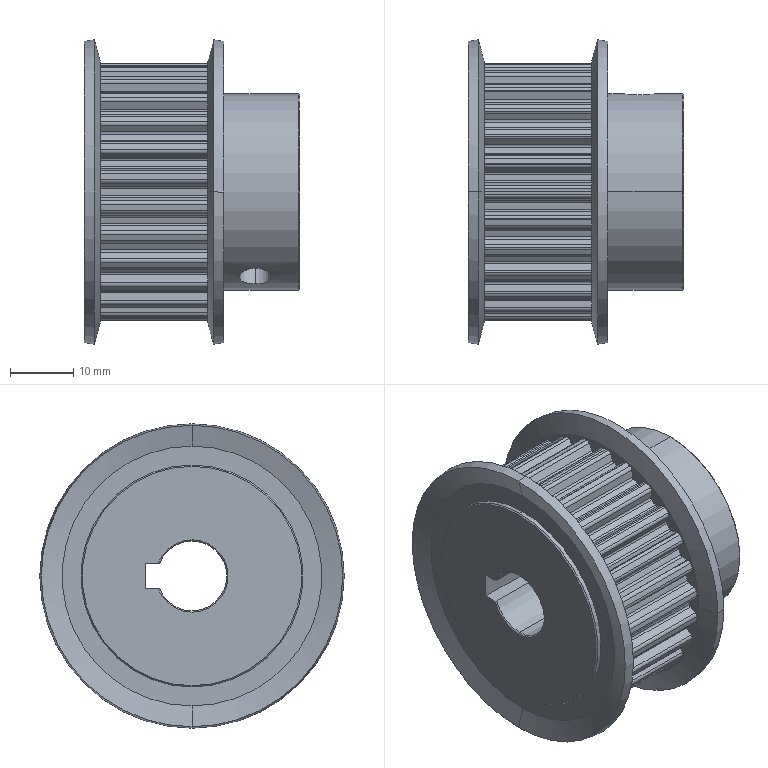Part | STEP file | Timing pulley TTPA26T5150-B-N11_MISUMI_TTPA26T5150-B-N11 | 1 solid | 292 faces | box 34 x 48 x 48 mm | volume 32918 mm3 | cylinder 197 | plane 65 | cone 30 | commonest cylinder face diameters 0.8 x62 1.2 x62 40.6 x27 37 x26 3.242 x4 5 x4